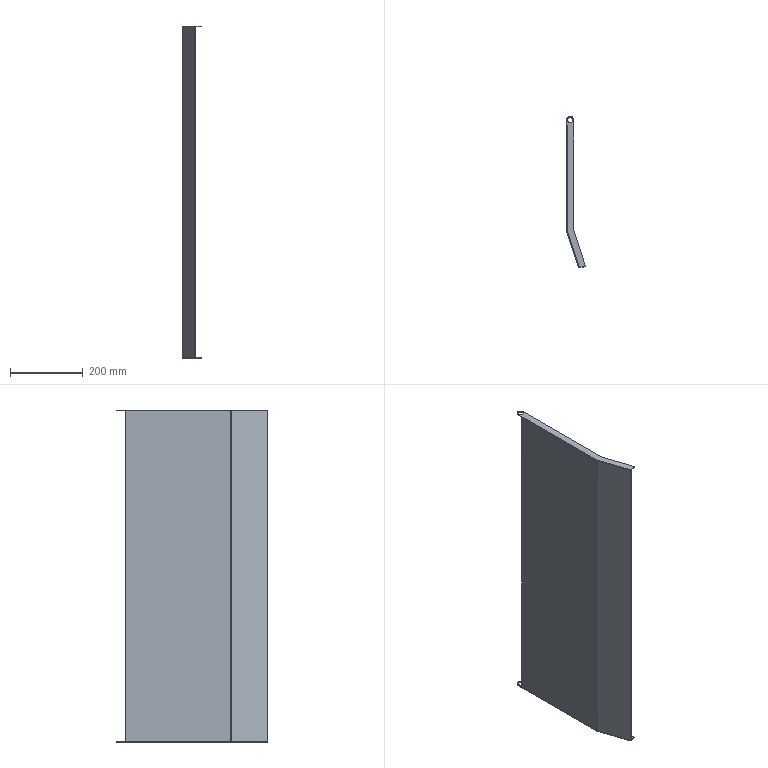Part | SolidWorks | features FlatPattern 2, SMBaseFlange 2, SheetMetal 2, ICE 1, MirrorSolid 1 | 2 solids | 46 faces | box 52.165 x 415.629 x 914 mm | volume 1472368 mm3 | plane 36 | cylinder 10 | commonest cylinder face diameters 15 x4 1.473 x2 5.473 x2 20 x2
STEP:
#1=CARTESIAN_POINT('',(0.5,405.,455.));
#2=VERTEX_POINT('',#1);
#3=CARTESIAN_POINT('',(15.5,405.,455.));
#4=VERTEX_POINT('',#3);
#5=CARTESIAN_POINT('',(8.,405.,455.));
#6=DIRECTION('',(0.,0.,1.));
#7=DIRECTION('',(1.,0.,0.));
#8=AXIS2_PLACEMENT_3D('',#5,#6,#7);
#9=CIRCLE('',#8,7.5);
#10=EDGE_CURVE('',#2,#4,#9,.T.);
#11=ORIENTED_EDGE('',*,*,#10,.F.);
#12=CARTESIAN_POINT('',(0.5,405.,457.));
#13=VERTEX_POINT('',#12);
#14=CARTESIAN_POINT('',(0.5,405.,455.));
#15=DIRECTION('',(0.,0.,1.));
#16=VECTOR('',#15,1000.);
#17=LINE('',#14,#16);
#18=EDGE_CURVE('',#2,#13,#17,.T.);
#19=ORIENTED_EDGE('',*,*,#18,.T.);
#20=CARTESIAN_POINT('',(15.5,405.,457.));
#21=VERTEX_POINT('',#20);
#22=CARTESIAN_POINT('',(8.,405.,457.));
#23=DIRECTION('',(0.,0.,1.));
#24=DIRECTION('',(1.,0.,0.));
#25=AXIS2_PLACEMENT_3D('',#22,#23,#24);
#26=CIRCLE('',#25,7.5);
#27=EDGE_CURVE('',#13,#21,#26,.T.);
#28=ORIENTED_EDGE('',*,*,#27,.T.);
#29=CARTESIAN_POINT('',(15.5,405.,455.));
#30=DIRECTION('',(0.,0.,1.));
#31=VECTOR('',#30,1000.);
#32=LINE('',#29,#31);
#33=EDGE_CURVE('',#4,#21,#32,.T.);
#34=ORIENTED_EDGE('',*,*,#33,.F.);
#35=EDGE_LOOP('',(#11,#19,#28,#34));
#36=FACE_OUTER_BOUND('',#35,.T.);
#37=CARTESIAN_POINT('',(8.,405.,455.));
#38=DIRECTION('',(0.,0.,1.));
#39=DIRECTION('',(1.,0.,0.));
#40=AXIS2_PLACEMENT_3D('',#37,#38,#39);
#41=CYLINDRICAL_SURFACE('',#40,7.5);
#42=ADVANCED_FACE('',(#36),#41,.F.);
#43=CARTESIAN_POINT('',(-2.,390.,455.));
#44=VERTEX_POINT('',#43);
#45=CARTESIAN_POINT('',(-2.,390.,-455.));
#46=VERTEX_POINT('',#45);
#47=CARTESIAN_POINT('',(-2.,390.,455.));
#48=DIRECTION('',(0.,0.,-1.));
#49=VECTOR('',#48,1000.);
#50=LINE('',#47,#49);
#51=EDGE_CURVE('',#44,#46,#50,.T.);
#52=ORIENTED_EDGE('',*,*,#51,.F.);
#53=CARTESIAN_POINT('',(0.,390.,455.));
#54=VERTEX_POINT('',#53);
#55=CARTESIAN_POINT('',(-2.,390.,455.));
#56=DIRECTION('',(1.,0.,0.));
#57=VECTOR('',#56,1000.);
#58=LINE('',#55,#57);
#59=EDGE_CURVE('',#44,#54,#58,.T.);
#60=ORIENTED_EDGE('',*,*,#59,.T.);
#61=CARTESIAN_POINT('',(0.,390.,-455.));
#62=VERTEX_POINT('',#61);
#63=CARTESIAN_POINT('',(0.,390.,455.));
#64=DIRECTION('',(0.,0.,-1.));
#65=VECTOR('',#64,1000.);
#66=LINE('',#63,#65);
#67=EDGE_CURVE('',#54,#62,#66,.T.);
#68=ORIENTED_EDGE('',*,*,#67,.T.);
#69=CARTESIAN_POINT('',(-2.,390.,-455.));
#70=DIRECTION('',(1.,0.,0.));
#71=VECTOR('',#70,1000.);
#72=LINE('',#69,#71);
#73=EDGE_CURVE('',#46,#62,#72,.T.);
#74=ORIENTED_EDGE('',*,*,#73,.F.);
#75=EDGE_LOOP('',(#52,#60,#68,#74));
#76=FACE_OUTER_BOUND('',#75,.T.);
#77=CARTESIAN_POINT('',(-2.,390.,455.));
#78=DIRECTION('',(0.,1.,0.));
#79=DIRECTION('',(0.,0.,1.));
#80=AXIS2_PLACEMENT_3D('',#77,#78,#79);
#81=PLANE('',#80);
#82=ADVANCED_FACE('',(#76),#81,.T.);
#83=CARTESIAN_POINT('',(-2.,100.119,455.));
#84=VERTEX_POINT('',#83);
#85=CARTESIAN_POINT('',(-1.861,99.258,455.));
#86=VERTEX_POINT('',#85);
#87=CARTESIAN_POINT('',(0.7366,100.119,455.));
#88=DIRECTION('',(0.,0.,1.));
#89=DIRECTION('',(1.,0.,0.));
#90=AXIS2_PLACEMENT_3D('',#87,#88,#89);
#91=CIRCLE('',#90,2.737);
#92=EDGE_CURVE('',#84,#86,#91,.T.);
#93=ORIENTED_EDGE('',*,*,#92,.T.);
#94=CARTESIAN_POINT('',(-1.862,100.119,455.));
#95=VERTEX_POINT('',#94);
#96=CARTESIAN_POINT('',(-1.861,99.258,455.));
#97=DIRECTION('',(0.0004776,-1.,0.));
#98=VECTOR('',#97,1000.);
#99=LINE('',#96,#98);
#100=EDGE_CURVE('',#95,#86,#99,.T.);
#101=ORIENTED_EDGE('',*,*,#100,.F.);
#102=CARTESIAN_POINT('',(-2.,100.119,455.));
#103=DIRECTION('',(1.,0.,0.));
#104=VECTOR('',#103,1000.);
#105=LINE('',#102,#104);
#106=EDGE_CURVE('',#84,#95,#105,.T.);
#107=ORIENTED_EDGE('',*,*,#106,.F.);
#108=EDGE_LOOP('',(#93,#101,#107));
#109=FACE_OUTER_BOUND('',#108,.T.);
#110=CARTESIAN_POINT('',(0.03738,99.887,455.));
#111=DIRECTION('',(0.,0.,1.));
#112=DIRECTION('',(1.,0.,0.));
#113=AXIS2_PLACEMENT_3D('',#110,#111,#112);
#114=PLANE('',#113);
#115=ADVANCED_FACE('',(#109),#114,.T.);
#116=CARTESIAN_POINT('',(-1.861,99.258,455.));
#117=DIRECTION('',(0.0004776,-1.,0.));
#118=VECTOR('',#117,1000.);
#119=LINE('',#116,#118);
#120=EDGE_CURVE('',#44,#95,#119,.T.);
#121=ORIENTED_EDGE('',*,*,#120,.F.);
#122=CARTESIAN_POINT('',(-2.,390.,455.));
#123=DIRECTION('',(0.,-1.,0.));
#124=VECTOR('',#123,1000.);
#125=LINE('',#122,#124);
#126=EDGE_CURVE('',#44,#84,#125,.T.);
#127=ORIENTED_EDGE('',*,*,#126,.T.);
#128=ORIENTED_EDGE('',*,*,#106,.T.);
#129=EDGE_LOOP('',(#121,#127,#128));
#130=FACE_OUTER_BOUND('',#129,.T.);
#131=CARTESIAN_POINT('',(0.7366,100.119,455.));
#132=DIRECTION('',(0.,0.,-1.));
#133=DIRECTION('',(-1.,0.,0.));
#134=AXIS2_PLACEMENT_3D('',#131,#132,#133);
#135=PLANE('',#134);
#136=ADVANCED_FACE('',(#130),#135,.F.);
#137=CARTESIAN_POINT('',(0.,100.119,-455.));
#138=VERTEX_POINT('',#137);
#139=CARTESIAN_POINT('',(-2.,100.119,-455.));
#140=VERTEX_POINT('',#139);
#141=CARTESIAN_POINT('',(0.,100.119,-455.));
#142=DIRECTION('',(-1.,0.,0.));
#143=VECTOR('',#142,1000.);
#144=LINE('',#141,#143);
#145=EDGE_CURVE('',#138,#140,#144,.T.);
#146=ORIENTED_EDGE('',*,*,#145,.F.);
#147=CARTESIAN_POINT('',(0.03738,99.887,-455.));
#148=VERTEX_POINT('',#147);
#149=CARTESIAN_POINT('',(0.7366,100.119,-455.));
#150=DIRECTION('',(0.,0.,1.));
#151=DIRECTION('',(-1.,0.,0.));
#152=AXIS2_PLACEMENT_3D('',#149,#150,#151);
#153=CIRCLE('',#152,0.7366);
#154=EDGE_CURVE('',#138,#148,#153,.T.);
#155=ORIENTED_EDGE('',*,*,#154,.T.);
#156=CARTESIAN_POINT('',(-1.861,99.258,-455.));
#157=VERTEX_POINT('',#156);
#158=CARTESIAN_POINT('',(-1.861,99.258,-455.));
#159=DIRECTION('',(0.9493,0.3145,0.));
#160=VECTOR('',#159,1000.);
#161=LINE('',#158,#160);
#162=EDGE_CURVE('',#157,#148,#161,.T.);
#163=ORIENTED_EDGE('',*,*,#162,.F.);
#164=CARTESIAN_POINT('',(0.7366,100.119,-455.));
#165=DIRECTION('',(0.,0.,1.));
#166=DIRECTION('',(1.,0.,0.));
#167=AXIS2_PLACEMENT_3D('',#164,#165,#166);
#168=CIRCLE('',#167,2.737);
#169=EDGE_CURVE('',#140,#157,#168,.T.);
#170=ORIENTED_EDGE('',*,*,#169,.F.);
#171=EDGE_LOOP('',(#146,#155,#163,#170));
#172=FACE_OUTER_BOUND('',#171,.T.);
#173=CARTESIAN_POINT('',(0.,100.119,-455.));
#174=DIRECTION('',(0.,0.,-1.));
#175=DIRECTION('',(-1.,0.,0.));
#176=AXIS2_PLACEMENT_3D('',#173,#174,#175);
#177=PLANE('',#176);
#178=ADVANCED_FACE('',(#172),#177,.T.);
#179=CARTESIAN_POINT('',(0.,390.,-455.));
#180=DIRECTION('',(0.,-1.,0.));
#181=VECTOR('',#180,1000.);
#182=LINE('',#179,#181);
#183=EDGE_CURVE('',#62,#138,#182,.T.);
#184=ORIENTED_EDGE('',*,*,#183,.T.);
#185=ORIENTED_EDGE('',*,*,#145,.T.);
#186=CARTESIAN_POINT('',(-2.,390.,-455.));
#187=DIRECTION('',(0.,-1.,0.));
#188=VECTOR('',#187,1000.);
#189=LINE('',#186,#188);
#190=EDGE_CURVE('',#46,#140,#189,.T.);
#191=ORIENTED_EDGE('',*,*,#190,.F.);
#192=ORIENTED_EDGE('',*,*,#73,.T.);
#193=EDGE_LOOP('',(#184,#185,#191,#192));
#194=FACE_OUTER_BOUND('',#193,.T.);
#195=CARTESIAN_POINT('',(-1.861,99.258,-455.));
#196=DIRECTION('',(0.,0.,-1.));
#197=DIRECTION('',(-1.,0.,0.));
#198=AXIS2_PLACEMENT_3D('',#195,#196,#197);
#199=PLANE('',#198);
#200=ADVANCED_FACE('',(#194),#199,.T.);
#201=CARTESIAN_POINT('',(31.233,-0.629,-455.));
#202=VERTEX_POINT('',#201);
#203=CARTESIAN_POINT('',(-1.899,99.371,-455.));
#204=DIRECTION('',(0.3145,-0.9493,0.));
#205=VECTOR('',#204,1000.);
#206=LINE('',#203,#205);
#207=EDGE_CURVE('',#157,#202,#206,.T.);
#208=ORIENTED_EDGE('',*,*,#207,.T.);
#209=CARTESIAN_POINT('',(31.233,-0.629,455.));
#210=VERTEX_POINT('',#209);
#211=CARTESIAN_POINT('',(31.233,-0.629,455.));
#212=DIRECTION('',(0.,0.,-1.));
#213=VECTOR('',#212,1000.);
#214=LINE('',#211,#213);
#215=EDGE_CURVE('',#210,#202,#214,.T.);
#216=ORIENTED_EDGE('',*,*,#215,.F.);
#217=CARTESIAN_POINT('',(31.233,-0.629,457.));
#218=VERTEX_POINT('',#217);
#219=CARTESIAN_POINT('',(31.233,-0.629,457.));
#220=DIRECTION('',(0.,0.,-1.));
#221=VECTOR('',#220,1000.);
#222=LINE('',#219,#221);
#223=EDGE_CURVE('',#218,#210,#222,.T.);
#224=ORIENTED_EDGE('',*,*,#223,.F.);
#225=CARTESIAN_POINT('',(-1.861,99.258,457.));
#226=VERTEX_POINT('',#225);
#227=CARTESIAN_POINT('',(31.233,-0.629,457.));
#228=DIRECTION('',(0.3145,-0.9493,0.));
#229=VECTOR('',#228,1000.);
#230=LINE('',#227,#229);
#231=EDGE_CURVE('',#226,#218,#230,.T.);
#232=ORIENTED_EDGE('',*,*,#231,.F.);
#233=CARTESIAN_POINT('',(-1.861,99.258,457.));
#234=DIRECTION('',(0.,0.,-1.));
#235=VECTOR('',#234,1000.);
#236=LINE('',#233,#235);
#237=EDGE_CURVE('',#226,#86,#236,.T.);
#238=ORIENTED_EDGE('',*,*,#237,.T.);
#239=CARTESIAN_POINT('',(-1.861,99.258,455.));
#240=DIRECTION('',(0.,0.,-1.));
#241=VECTOR('',#240,1000.);
#242=LINE('',#239,#241);
#243=EDGE_CURVE('',#86,#157,#242,.T.);
#244=ORIENTED_EDGE('',*,*,#243,.T.);
#245=EDGE_LOOP('',(#208,#216,#224,#232,#238,#244));
#246=FACE_OUTER_BOUND('',#245,.T.);
#247=CARTESIAN_POINT('',(-1.899,99.371,455.));
#248=DIRECTION('',(0.9493,0.3145,0.));
#249=DIRECTION('',(-0.3145,0.9493,0.));
#250=AXIS2_PLACEMENT_3D('',#247,#248,#249);
#251=PLANE('',#250);
#252=ADVANCED_FACE('',(#246),#251,.F.);
#253=CARTESIAN_POINT('',(33.132,0.,-455.));
#254=VERTEX_POINT('',#253);
#255=CARTESIAN_POINT('',(33.132,0.,-455.));
#256=DIRECTION('',(-0.9493,-0.3145,0.));
#257=VECTOR('',#256,1000.);
#258=LINE('',#255,#257);
#259=EDGE_CURVE('',#254,#202,#258,.T.);
#260=ORIENTED_EDGE('',*,*,#259,.F.);
#261=CARTESIAN_POINT('',(33.132,0.,455.));
#262=VERTEX_POINT('',#261);
#263=CARTESIAN_POINT('',(33.132,0.,455.));
#264=DIRECTION('',(0.,0.,-1.));
#265=VECTOR('',#264,1000.);
#266=LINE('',#263,#265);
#267=EDGE_CURVE('',#262,#254,#266,.T.);
#268=ORIENTED_EDGE('',*,*,#267,.F.);
#269=CARTESIAN_POINT('',(33.132,0.,455.));
#270=DIRECTION('',(-0.9493,-0.3145,0.));
#271=VECTOR('',#270,1000.);
#272=LINE('',#269,#271);
#273=EDGE_CURVE('',#262,#210,#272,.T.);
#274=ORIENTED_EDGE('',*,*,#273,.T.);
#275=ORIENTED_EDGE('',*,*,#215,.T.);
#276=EDGE_LOOP('',(#260,#268,#274,#275));
#277=FACE_OUTER_BOUND('',#276,.T.);
#278=CARTESIAN_POINT('',(33.132,0.,455.));
#279=DIRECTION('',(0.3145,-0.9493,0.));
#280=DIRECTION('',(0.9493,0.3145,0.));
#281=AXIS2_PLACEMENT_3D('',#278,#279,#280);
#282=PLANE('',#281);
#283=ADVANCED_FACE('',(#277),#282,.T.);
#284=CARTESIAN_POINT('',(0.,100.,-455.));
#285=DIRECTION('',(0.3145,-0.9493,0.));
#286=VECTOR('',#285,1000.);
#287=LINE('',#284,#286);
#288=EDGE_CURVE('',#148,#254,#287,.T.);
#289=ORIENTED_EDGE('',*,*,#288,.F.);
#290=CARTESIAN_POINT('',(0.03738,99.887,455.));
#291=VERTEX_POINT('',#290);
#292=CARTESIAN_POINT('',(0.03738,99.887,455.));
#293=DIRECTION('',(0.,0.,-1.));
#294=VECTOR('',#293,1000.);
#295=LINE('',#292,#294);
#296=EDGE_CURVE('',#291,#148,#295,.T.);
#297=ORIENTED_EDGE('',*,*,#296,.F.);
#298=CARTESIAN_POINT('',(0.,100.,455.));
#299=DIRECTION('',(0.3145,-0.9493,0.));
#300=VECTOR('',#299,1000.);
#301=LINE('',#298,#300);
#302=EDGE_CURVE('',#291,#262,#301,.T.);
#303=ORIENTED_EDGE('',*,*,#302,.T.);
#304=ORIENTED_EDGE('',*,*,#267,.T.);
#305=EDGE_LOOP('',(#289,#297,#303,#304));
#306=FACE_OUTER_BOUND('',#305,.T.);
#307=CARTESIAN_POINT('',(0.,100.,455.));
#308=DIRECTION('',(0.9493,0.3145,0.));
#309=DIRECTION('',(-0.3145,0.9493,0.));
#310=AXIS2_PLACEMENT_3D('',#307,#308,#309);
#311=PLANE('',#310);
#312=ADVANCED_FACE('',(#306),#311,.T.);
#313=ORIENTED_EDGE('',*,*,#154,.F.);
#314=CARTESIAN_POINT('',(0.,100.119,455.));
#315=VERTEX_POINT('',#314);
#316=CARTESIAN_POINT('',(0.,100.119,455.));
#317=DIRECTION('',(0.,0.,-1.));
#318=VECTOR('',#317,1000.);
#319=LINE('',#316,#318);
#320=EDGE_CURVE('',#315,#138,#319,.T.);
#321=ORIENTED_EDGE('',*,*,#320,.F.);
#322=CARTESIAN_POINT('',(0.7366,100.119,455.));
#323=DIRECTION('',(0.,0.,1.));
#324=DIRECTION('',(-1.,0.,0.));
#325=AXIS2_PLACEMENT_3D('',#322,#323,#324);
#326=CIRCLE('',#325,0.7366);
#327=EDGE_CURVE('',#315,#291,#326,.T.);
#328=ORIENTED_EDGE('',*,*,#327,.T.);
#329=ORIENTED_EDGE('',*,*,#296,.T.);
#330=EDGE_LOOP('',(#313,#321,#328,#329));
#331=FACE_OUTER_BOUND('',#330,.T.);
#332=CARTESIAN_POINT('',(0.7366,100.119,455.));
#333=DIRECTION('',(0.,0.,-1.));
#334=DIRECTION('',(-1.,0.,0.));
#335=AXIS2_PLACEMENT_3D('',#332,#333,#334);
#336=CYLINDRICAL_SURFACE('',#335,0.7366);
#337=ADVANCED_FACE('',(#331),#336,.F.);
#338=ORIENTED_EDGE('',*,*,#183,.F.);
#339=ORIENTED_EDGE('',*,*,#67,.F.);
#340=CARTESIAN_POINT('',(0.,390.,455.));
#341=DIRECTION('',(0.,-1.,0.));
#342=VECTOR('',#341,1000.);
#343=LINE('',#340,#342);
#344=EDGE_CURVE('',#54,#315,#343,.T.);
#345=ORIENTED_EDGE('',*,*,#344,.T.);
#346=ORIENTED_EDGE('',*,*,#320,.T.);
#347=EDGE_LOOP('',(#338,#339,#345,#346));
#348=FACE_OUTER_BOUND('',#347,.T.);
#349=CARTESIAN_POINT('',(0.,390.,455.));
#350=DIRECTION('',(1.,0.,0.));
#351=DIRECTION('',(0.,1.,0.));
#352=AXIS2_PLACEMENT_3D('',#349,#350,#351);
#353=PLANE('',#352);
#354=ADVANCED_FACE('',(#348),#353,.T.);
#355=ORIENTED_EDGE('',*,*,#190,.T.);
#356=CARTESIAN_POINT('',(-2.,100.119,455.));
#357=DIRECTION('',(0.,0.,-1.));
#358=VECTOR('',#357,1000.);
#359=LINE('',#356,#358);
#360=EDGE_CURVE('',#84,#140,#359,.T.);
#361=ORIENTED_EDGE('',*,*,#360,.F.);
#362=ORIENTED_EDGE('',*,*,#126,.F.);
#363=ORIENTED_EDGE('',*,*,#51,.T.);
#364=EDGE_LOOP('',(#355,#361,#362,#363));
#365=FACE_OUTER_BOUND('',#364,.T.);
#366=CARTESIAN_POINT('',(-2.,390.,455.));
#367=DIRECTION('',(1.,0.,0.));
#368=DIRECTION('',(0.,1.,0.));
#369=AXIS2_PLACEMENT_3D('',#366,#367,#368);
#370=PLANE('',#369);
#371=ADVANCED_FACE('',(#365),#370,.F.);
#372=ORIENTED_EDGE('',*,*,#169,.T.);
#373=ORIENTED_EDGE('',*,*,#243,.F.);
#374=ORIENTED_EDGE('',*,*,#92,.F.);
#375=ORIENTED_EDGE('',*,*,#360,.T.);
#376=EDGE_LOOP('',(#372,#373,#374,#375));
#377=FACE_OUTER_BOUND('',#376,.T.);
#378=CARTESIAN_POINT('',(0.7366,100.119,455.));
#379=DIRECTION('',(0.,0.,-1.));
#380=DIRECTION('',(-1.,0.,0.));
#381=AXIS2_PLACEMENT_3D('',#378,#379,#380);
#382=CYLINDRICAL_SURFACE('',#381,2.737);
#383=ADVANCED_FACE('',(#377),#382,.T.);
#384=ORIENTED_EDGE('',*,*,#207,.F.);
#385=ORIENTED_EDGE('',*,*,#162,.T.);
#386=ORIENTED_EDGE('',*,*,#288,.T.);
#387=ORIENTED_EDGE('',*,*,#259,.T.);
#388=EDGE_LOOP('',(#384,#385,#386,#387));
#389=FACE_OUTER_BOUND('',#388,.T.);
#390=CARTESIAN_POINT('',(0.7366,100.119,-455.));
#391=DIRECTION('',(0.,0.,-1.));
#392=DIRECTION('',(-1.,0.,0.));
#393=AXIS2_PLACEMENT_3D('',#390,#391,#392);
#394=PLANE('',#393);
#395=ADVANCED_FACE('',(#389),#394,.T.);
#396=ORIENTED_EDGE('',*,*,#273,.F.);
#397=ORIENTED_EDGE('',*,*,#302,.F.);
#398=ORIENTED_EDGE('',*,*,#327,.F.);
#399=ORIENTED_EDGE('',*,*,#344,.F.);
#400=ORIENTED_EDGE('',*,*,#59,.F.);
#401=CARTESIAN_POINT('',(-2.,405.,455.));
#402=VERTEX_POINT('',#401);
#403=CARTESIAN_POINT('',(-2.,390.,455.));
#404=DIRECTION('',(0.,-1.,0.));
#405=VECTOR('',#404,1000.);
#406=LINE('',#403,#405);
#407=EDGE_CURVE('',#402,#44,#406,.T.);
#408=ORIENTED_EDGE('',*,*,#407,.F.);
#409=CARTESIAN_POINT('',(18.,405.,455.));
#410=VERTEX_POINT('',#409);
#411=CARTESIAN_POINT('',(8.,405.,455.));
#412=DIRECTION('',(0.,0.,1.));
#413=DIRECTION('',(1.,0.,0.));
#414=AXIS2_PLACEMENT_3D('',#411,#412,#413);
#415=CIRCLE('',#414,10.);
#416=EDGE_CURVE('',#410,#402,#415,.T.);
#417=ORIENTED_EDGE('',*,*,#416,.F.);
#418=CARTESIAN_POINT('',(18.,99.573,455.));
#419=VERTEX_POINT('',#418);
#420=CARTESIAN_POINT('',(18.,390.,455.));
#421=DIRECTION('',(0.,1.,0.));
#422=VECTOR('',#421,1000.);
#423=LINE('',#420,#422);
#424=EDGE_CURVE('',#419,#410,#423,.T.);
#425=ORIENTED_EDGE('',*,*,#424,.F.);
#426=CARTESIAN_POINT('',(50.165,2.49,455.));
#427=VERTEX_POINT('',#426);
#428=CARTESIAN_POINT('',(18.,99.573,455.));
#429=DIRECTION('',(-0.3145,0.9493,0.));
#430=VECTOR('',#429,1000.);
#431=LINE('',#428,#430);
#432=EDGE_CURVE('',#427,#419,#431,.T.);
#433=ORIENTED_EDGE('',*,*,#432,.F.);
#434=CARTESIAN_POINT('',(50.165,2.49,455.));
#435=DIRECTION('',(0.9867,0.1625,0.));
#436=VECTOR('',#435,1000.);
#437=LINE('',#434,#436);
#438=EDGE_CURVE('',#210,#427,#437,.T.);
#439=ORIENTED_EDGE('',*,*,#438,.F.);
#440=EDGE_LOOP('',(#396,#397,#398,#399,#400,#408,#417,#425,#433,#439));
#441=FACE_OUTER_BOUND('',#440,.T.);
#442=CARTESIAN_POINT('',(8.,405.,455.));
#443=DIRECTION('',(0.,0.,1.));
#444=DIRECTION('',(1.,0.,0.));
#445=AXIS2_PLACEMENT_3D('',#442,#443,#444);
#446=CIRCLE('',#445,7.5);
#447=EDGE_CURVE('',#4,#2,#446,.T.);
#448=ORIENTED_EDGE('',*,*,#447,.T.);
#449=ORIENTED_EDGE('',*,*,#10,.T.);
#450=EDGE_LOOP('',(#448,#449));
#451=FACE_BOUND('',#450,.T.);
#452=CARTESIAN_POINT('',(0.,0.,455.));
#453=DIRECTION('',(0.,0.,1.));
#454=DIRECTION('',(1.,0.,0.));
#455=AXIS2_PLACEMENT_3D('',#452,#453,#454);
#456=PLANE('',#455);
#457=ADVANCED_FACE('',(#441,#451),#456,.F.);
#458=ORIENTED_EDGE('',*,*,#424,.T.);
#459=CARTESIAN_POINT('',(18.,405.,457.));
#460=VERTEX_POINT('',#459);
#461=CARTESIAN_POINT('',(18.,405.,455.));
#462=DIRECTION('',(0.,0.,1.));
#463=VECTOR('',#462,1000.);
#464=LINE('',#461,#463);
#465=EDGE_CURVE('',#410,#460,#464,.T.);
#466=ORIENTED_EDGE('',*,*,#465,.T.);
#467=CARTESIAN_POINT('',(18.,99.573,457.));
#468=VERTEX_POINT('',#467);
#469=CARTESIAN_POINT('',(18.,390.,457.));
#470=DIRECTION('',(0.,1.,0.));
#471=VECTOR('',#470,1000.);
#472=LINE('',#469,#471);
#473=EDGE_CURVE('',#468,#460,#472,.T.);
#474=ORIENTED_EDGE('',*,*,#473,.F.);
#475=CARTESIAN_POINT('',(18.,99.573,457.));
#476=DIRECTION('',(0.,0.,-1.));
#477=VECTOR('',#476,1000.);
#478=LINE('',#475,#477);
#479=EDGE_CURVE('',#468,#419,#478,.T.);
#480=ORIENTED_EDGE('',*,*,#479,.T.);
#481=EDGE_LOOP('',(#458,#466,#474,#480));
#482=FACE_OUTER_BOUND('',#481,.T.);
#483=CARTESIAN_POINT('',(18.,390.,457.));
#484=DIRECTION('',(-1.,0.,0.));
#485=DIRECTION('',(0.,-1.,0.));
#486=AXIS2_PLACEMENT_3D('',#483,#484,#485);
#487=PLANE('',#486);
#488=ADVANCED_FACE('',(#482),#487,.F.);
#489=ORIENTED_EDGE('',*,*,#120,.T.);
#490=ORIENTED_EDGE('',*,*,#100,.T.);
#491=ORIENTED_EDGE('',*,*,#237,.F.);
#492=CARTESIAN_POINT('',(-2.,390.,457.));
#493=VERTEX_POINT('',#492);
#494=CARTESIAN_POINT('',(-1.861,99.258,457.));
#495=DIRECTION('',(0.0004776,-1.,0.));
#496=VECTOR('',#495,1000.);
#497=LINE('',#494,#496);
#498=EDGE_CURVE('',#493,#226,#497,.T.);
#499=ORIENTED_EDGE('',*,*,#498,.F.);
#500=CARTESIAN_POINT('',(-2.,390.,457.));
#501=DIRECTION('',(0.,0.,-1.));
#502=VECTOR('',#501,1000.);
#503=LINE('',#500,#502);
#504=EDGE_CURVE('',#493,#44,#503,.T.);
#505=ORIENTED_EDGE('',*,*,#504,.T.);
#506=EDGE_LOOP('',(#489,#490,#491,#499,#505));
#507=FACE_OUTER_BOUND('',#506,.T.);
#508=CARTESIAN_POINT('',(-1.861,99.258,457.));
#509=DIRECTION('',(1.,0.0004776,0.));
#510=DIRECTION('',(-0.0004776,1.,0.));
#511=AXIS2_PLACEMENT_3D('',#508,#509,#510);
#512=PLANE('',#511);
#513=ADVANCED_FACE('',(#507),#512,.F.);
#514=ORIENTED_EDGE('',*,*,#438,.T.);
#515=CARTESIAN_POINT('',(50.165,2.49,457.));
#516=VERTEX_POINT('',#515);
#517=CARTESIAN_POINT('',(50.165,2.49,457.));
#518=DIRECTION('',(0.,0.,-1.));
#519=VECTOR('',#518,1000.);
#520=LINE('',#517,#519);
#521=EDGE_CURVE('',#516,#427,#520,.T.);
#522=ORIENTED_EDGE('',*,*,#521,.F.);
#523=CARTESIAN_POINT('',(50.165,2.49,457.));
#524=DIRECTION('',(0.9867,0.1625,0.));
#525=VECTOR('',#524,1000.);
#526=LINE('',#523,#525);
#527=EDGE_CURVE('',#218,#516,#526,.T.);
#528=ORIENTED_EDGE('',*,*,#527,.F.);
#529=ORIENTED_EDGE('',*,*,#223,.T.);
#530=EDGE_LOOP('',(#514,#522,#528,#529));
#531=FACE_OUTER_BOUND('',#530,.T.);
#532=CARTESIAN_POINT('',(50.165,2.49,457.));
#533=DIRECTION('',(-0.1625,0.9867,0.));
#534=DIRECTION('',(-0.9867,-0.1625,0.));
#535=AXIS2_PLACEMENT_3D('',#532,#533,#534);
#536=PLANE('',#535);
#537=ADVANCED_FACE('',(#531),#536,.F.);
#538=ORIENTED_EDGE('',*,*,#432,.T.);
#539=ORIENTED_EDGE('',*,*,#479,.F.);
#540=CARTESIAN_POINT('',(18.,99.573,457.));
#541=DIRECTION('',(-0.3145,0.9493,0.));
#542=VECTOR('',#541,1000.);
#543=LINE('',#540,#542);
#544=EDGE_CURVE('',#516,#468,#543,.T.);
#545=ORIENTED_EDGE('',*,*,#544,.F.);
#546=ORIENTED_EDGE('',*,*,#521,.T.);
#547=EDGE_LOOP('',(#538,#539,#545,#546));
#548=FACE_OUTER_BOUND('',#547,.T.);
#549=CARTESIAN_POINT('',(18.,99.573,457.));
#550=DIRECTION('',(-0.9493,-0.3145,0.));
#551=DIRECTION('',(0.3145,-0.9493,0.));
#552=AXIS2_PLACEMENT_3D('',#549,#550,#551);
#553=PLANE('',#552);
#554=ADVANCED_FACE('',(#548),#553,.F.);
#555=ORIENTED_EDGE('',*,*,#473,.T.);
#556=CARTESIAN_POINT('',(-2.,405.,457.));
#557=VERTEX_POINT('',#556);
#558=CARTESIAN_POINT('',(8.,405.,457.));
#559=DIRECTION('',(0.,0.,1.));
#560=DIRECTION('',(1.,0.,0.));
#561=AXIS2_PLACEMENT_3D('',#558,#559,#560);
#562=CIRCLE('',#561,10.);
#563=EDGE_CURVE('',#460,#557,#562,.T.);
#564=ORIENTED_EDGE('',*,*,#563,.T.);
#565=CARTESIAN_POINT('',(-2.,390.,457.));
#566=DIRECTION('',(0.,-1.,0.));
#567=VECTOR('',#566,1000.);
#568=LINE('',#565,#567);
#569=EDGE_CURVE('',#557,#493,#568,.T.);
#570=ORIENTED_EDGE('',*,*,#569,.T.);
#571=ORIENTED_EDGE('',*,*,#498,.T.);
#572=ORIENTED_EDGE('',*,*,#231,.T.);
#573=ORIENTED_EDGE('',*,*,#527,.T.);
#574=ORIENTED_EDGE('',*,*,#544,.T.);
#575=EDGE_LOOP('',(#555,#564,#570,#571,#572,#573,#574));
#576=FACE_OUTER_BOUND('',#575,.T.);
#577=CARTESIAN_POINT('',(8.,405.,457.));
#578=DIRECTION('',(0.,0.,1.));
#579=DIRECTION('',(1.,0.,0.));
#580=AXIS2_PLACEMENT_3D('',#577,#578,#579);
#581=CIRCLE('',#580,7.5);
#582=EDGE_CURVE('',#21,#13,#581,.T.);
#583=ORIENTED_EDGE('',*,*,#582,.F.);
#584=ORIENTED_EDGE('',*,*,#27,.F.);
#585=EDGE_LOOP('',(#583,#584));
#586=FACE_BOUND('',#585,.T.);
#587=CARTESIAN_POINT('',(0.,0.,457.));
#588=DIRECTION('',(0.,0.,1.));
#589=DIRECTION('',(1.,0.,0.));
#590=AXIS2_PLACEMENT_3D('',#587,#588,#589);
#591=PLANE('',#590);
#592=ADVANCED_FACE('',(#576,#586),#591,.T.);
#593=ORIENTED_EDGE('',*,*,#569,.F.);
#594=CARTESIAN_POINT('',(-2.,405.,455.));
#595=DIRECTION('',(0.,0.,1.));
#596=VECTOR('',#595,1000.);
#597=LINE('',#594,#596);
#598=EDGE_CURVE('',#402,#557,#597,.T.);
#599=ORIENTED_EDGE('',*,*,#598,.F.);
#600=ORIENTED_EDGE('',*,*,#407,.T.);
#601=ORIENTED_EDGE('',*,*,#504,.F.);
#602=EDGE_LOOP('',(#593,#599,#600,#601));
#603=FACE_OUTER_BOUND('',#602,.T.);
#604=CARTESIAN_POINT('',(-2.,390.,455.));
#605=DIRECTION('',(-1.,0.,0.));
#606=DIRECTION('',(0.,0.,1.));
#607=AXIS2_PLACEMENT_3D('',#604,#605,#606);
#608=PLANE('',#607);
#609=ADVANCED_FACE('',(#603),#608,.T.);
#610=ORIENTED_EDGE('',*,*,#563,.F.);
#611=ORIENTED_EDGE('',*,*,#465,.F.);
#612=ORIENTED_EDGE('',*,*,#416,.T.);
#613=ORIENTED_EDGE('',*,*,#598,.T.);
#614=EDGE_LOOP('',(#610,#611,#612,#613));
#615=FACE_OUTER_BOUND('',#614,.T.);
#616=CARTESIAN_POINT('',(8.,405.,455.));
#617=DIRECTION('',(0.,0.,1.));
#618=DIRECTION('',(1.,0.,0.));
#619=AXIS2_PLACEMENT_3D('',#616,#617,#618);
#620=CYLINDRICAL_SURFACE('',#619,10.);
#621=ADVANCED_FACE('',(#615),#620,.T.);
#622=ORIENTED_EDGE('',*,*,#18,.F.);
#623=ORIENTED_EDGE('',*,*,#447,.F.);
#624=ORIENTED_EDGE('',*,*,#33,.T.);
#625=ORIENTED_EDGE('',*,*,#582,.T.);
#626=EDGE_LOOP('',(#622,#623,#624,#625));
#627=FACE_OUTER_BOUND('',#626,.T.);
#628=CARTESIAN_POINT('',(8.,405.,455.));
#629=DIRECTION('',(0.,0.,1.));
#630=DIRECTION('',(1.,0.,0.));
#631=AXIS2_PLACEMENT_3D('',#628,#629,#630);
#632=CYLINDRICAL_SURFACE('',#631,7.5);
#633=ADVANCED_FACE('',(#627),#632,.F.);
#634=CLOSED_SHELL('',(#42,#82,#115,#136,#178,#200,#252,#283,#312,#337,#354,#371,#383,#395,#457,#488,#513,#537,#554,#592,#609,#621,#633));
#635=MANIFOLD_SOLID_BREP('',#634);
#636=CARTESIAN_POINT('',(15.5,405.,-455.));
#637=VERTEX_POINT('',#636);
#638=CARTESIAN_POINT('',(0.5,405.,-455.));
#639=VERTEX_POINT('',#638);
#640=CARTESIAN_POINT('',(8.,405.,-455.));
#641=DIRECTION('',(0.,0.,1.));
#642=DIRECTION('',(1.,0.,0.));
#643=AXIS2_PLACEMENT_3D('',#640,#641,#642);
#644=CIRCLE('',#643,7.5);
#645=EDGE_CURVE('',#637,#639,#644,.T.);
#646=ORIENTED_EDGE('',*,*,#645,.T.);
#647=CARTESIAN_POINT('',(0.5,405.,-457.));
#648=VERTEX_POINT('',#647);
#649=CARTESIAN_POINT('',(0.5,405.,-455.));
#650=DIRECTION('',(0.,0.,-1.));
#651=VECTOR('',#650,1000.);
#652=LINE('',#649,#651);
#653=EDGE_CURVE('',#639,#648,#652,.T.);
#654=ORIENTED_EDGE('',*,*,#653,.T.);
#655=CARTESIAN_POINT('',(15.5,405.,-457.));
#656=VERTEX_POINT('',#655);
#657=CARTESIAN_POINT('',(8.,405.,-457.));
#658=DIRECTION('',(0.,0.,1.));
#659=DIRECTION('',(1.,0.,0.));
#660=AXIS2_PLACEMENT_3D('',#657,#658,#659);
#661=CIRCLE('',#660,7.5);
#662=EDGE_CURVE('',#656,#648,#661,.T.);
#663=ORIENTED_EDGE('',*,*,#662,.F.);
#664=CARTESIAN_POINT('',(15.5,405.,-455.));
#665=DIRECTION('',(0.,0.,-1.));
#666=VECTOR('',#665,1000.);
#667=LINE('',#664,#666);
#668=EDGE_CURVE('',#637,#656,#667,.T.);
#669=ORIENTED_EDGE('',*,*,#668,.F.);
#670=EDGE_LOOP('',(#646,#654,#663,#669));
#671=FACE_OUTER_BOUND('',#670,.T.);
#672=CARTESIAN_POINT('',(8.,405.,-455.));
#673=DIRECTION('',(0.,0.,-1.));
#674=DIRECTION('',(1.,0.,0.));
#675=AXIS2_PLACEMENT_3D('',#672,#673,#674);
#676=CYLINDRICAL_SURFACE('',#675,7.5);
#677=ADVANCED_FACE('',(#671),#676,.F.);
#678=CARTESIAN_POINT('',(-2.,390.,-455.));
#679=VERTEX_POINT('',#678);
#680=CARTESIAN_POINT('',(-2.,390.,455.));
#681=VERTEX_POINT('',#680);
#682=CARTESIAN_POINT('',(-2.,390.,-455.));
#683=DIRECTION('',(0.,0.,1.));
#684=VECTOR('',#683,1000.);
#685=LINE('',#682,#684);
#686=EDGE_CURVE('',#679,#681,#685,.T.);
#687=ORIENTED_EDGE('',*,*,#686,.T.);
#688=CARTESIAN_POINT('',(0.,390.,455.));
#689=VERTEX_POINT('',#688);
#690=CARTESIAN_POINT('',(-2.,390.,455.));
#691=DIRECTION('',(1.,0.,0.));
#692=VECTOR('',#691,1000.);
#693=LINE('',#690,#692);
#694=EDGE_CURVE('',#681,#689,#693,.T.);
#695=ORIENTED_EDGE('',*,*,#694,.T.);
#696=CARTESIAN_POINT('',(0.,390.,-455.));
#697=VERTEX_POINT('',#696);
#698=CARTESIAN_POINT('',(0.,390.,-455.));
#699=DIRECTION('',(0.,0.,1.));
#700=VECTOR('',#699,1000.);
#701=LINE('',#698,#700);
#702=EDGE_CURVE('',#697,#689,#701,.T.);
#703=ORIENTED_EDGE('',*,*,#702,.F.);
#704=CARTESIAN_POINT('',(-2.,390.,-455.));
#705=DIRECTION('',(1.,0.,0.));
#706=VECTOR('',#705,1000.);
#707=LINE('',#704,#706);
#708=EDGE_CURVE('',#679,#697,#707,.T.);
#709=ORIENTED_EDGE('',*,*,#708,.F.);
#710=EDGE_LOOP('',(#687,#695,#703,#709));
#711=FACE_OUTER_BOUND('',#710,.T.);
#712=CARTESIAN_POINT('',(-2.,390.,-455.));
#713=DIRECTION('',(0.,1.,0.));
#714=DIRECTION('',(0.,0.,-1.));
#715=AXIS2_PLACEMENT_3D('',#712,#713,#714);
#716=PLANE('',#715);
#717=ADVANCED_FACE('',(#711),#716,.T.);
#718=CARTESIAN_POINT('',(-2.,100.119,-455.));
#719=VERTEX_POINT('',#718);
#720=CARTESIAN_POINT('',(-1.861,99.258,-455.));
#721=VERTEX_POINT('',#720);
#722=CARTESIAN_POINT('',(0.7366,100.119,-455.));
#723=DIRECTION('',(0.,0.,1.));
#724=DIRECTION('',(1.,0.,0.));
#725=AXIS2_PLACEMENT_3D('',#722,#723,#724);
#726=CIRCLE('',#725,2.737);
#727=EDGE_CURVE('',#719,#721,#726,.T.);
#728=ORIENTED_EDGE('',*,*,#727,.F.);
#729=CARTESIAN_POINT('',(-1.862,100.119,-455.));
#730=VERTEX_POINT('',#729);
#731=CARTESIAN_POINT('',(-2.,100.119,-455.));
#732=DIRECTION('',(1.,0.,0.));
#733=VECTOR('',#732,1000.);
#734=LINE('',#731,#733);
#735=EDGE_CURVE('',#719,#730,#734,.T.);
#736=ORIENTED_EDGE('',*,*,#735,.T.);
#737=CARTESIAN_POINT('',(-1.861,99.258,-455.));
#738=DIRECTION('',(0.0004776,-1.,0.));
#739=VECTOR('',#738,1000.);
#740=LINE('',#737,#739);
#741=EDGE_CURVE('',#730,#721,#740,.T.);
#742=ORIENTED_EDGE('',*,*,#741,.T.);
#743=EDGE_LOOP('',(#728,#736,#742));
#744=FACE_OUTER_BOUND('',#743,.T.);
#745=CARTESIAN_POINT('',(0.03738,99.887,-455.));
#746=DIRECTION('',(0.,0.,-1.));
#747=DIRECTION('',(1.,0.,0.));
#748=AXIS2_PLACEMENT_3D('',#745,#746,#747);
#749=PLANE('',#748);
#750=ADVANCED_FACE('',(#744),#749,.T.);
#751=CARTESIAN_POINT('',(-1.861,99.258,-455.));
#752=DIRECTION('',(0.0004776,-1.,0.));
#753=VECTOR('',#752,1000.);
#754=LINE('',#751,#753);
#755=EDGE_CURVE('',#679,#730,#754,.T.);
#756=ORIENTED_EDGE('',*,*,#755,.T.);
#757=ORIENTED_EDGE('',*,*,#735,.F.);
#758=CARTESIAN_POINT('',(-2.,390.,-455.));
#759=DIRECTION('',(0.,-1.,0.));
#760=VECTOR('',#759,1000.);
#761=LINE('',#758,#760);
#762=EDGE_CURVE('',#679,#719,#761,.T.);
#763=ORIENTED_EDGE('',*,*,#762,.F.);
#764=EDGE_LOOP('',(#756,#757,#763));
#765=FACE_OUTER_BOUND('',#764,.T.);
#766=CARTESIAN_POINT('',(0.7366,100.119,-455.));
#767=DIRECTION('',(0.,0.,1.));
#768=DIRECTION('',(-1.,0.,0.));
#769=AXIS2_PLACEMENT_3D('',#766,#767,#768);
#770=PLANE('',#769);
#771=ADVANCED_FACE('',(#765),#770,.F.);
#772=CARTESIAN_POINT('',(0.,100.119,455.));
#773=VERTEX_POINT('',#772);
#774=CARTESIAN_POINT('',(-2.,100.119,455.));
#775=VERTEX_POINT('',#774);
#776=CARTESIAN_POINT('',(0.,100.119,455.));
#777=DIRECTION('',(-1.,0.,0.));
#778=VECTOR('',#777,1000.);
#779=LINE('',#776,#778);
#780=EDGE_CURVE('',#773,#775,#779,.T.);
#781=ORIENTED_EDGE('',*,*,#780,.T.);
#782=CARTESIAN_POINT('',(-1.861,99.258,455.));
#783=VERTEX_POINT('',#782);
#784=CARTESIAN_POINT('',(0.7366,100.119,455.));
#785=DIRECTION('',(0.,0.,1.));
#786=DIRECTION('',(1.,0.,0.));
#787=AXIS2_PLACEMENT_3D('',#784,#785,#786);
#788=CIRCLE('',#787,2.737);
#789=EDGE_CURVE('',#775,#783,#788,.T.);
#790=ORIENTED_EDGE('',*,*,#789,.T.);
#791=CARTESIAN_POINT('',(0.03738,99.887,455.));
#792=VERTEX_POINT('',#791);
#793=CARTESIAN_POINT('',(-1.861,99.258,455.));
#794=DIRECTION('',(0.9493,0.3145,0.));
#795=VECTOR('',#794,1000.);
#796=LINE('',#793,#795);
#797=EDGE_CURVE('',#783,#792,#796,.T.);
#798=ORIENTED_EDGE('',*,*,#797,.T.);
#799=CARTESIAN_POINT('',(0.7366,100.119,455.));
#800=DIRECTION('',(0.,0.,1.));
#801=DIRECTION('',(-1.,0.,0.));
#802=AXIS2_PLACEMENT_3D('',#799,#800,#801);
#803=CIRCLE('',#802,0.7366);
#804=EDGE_CURVE('',#773,#792,#803,.T.);
#805=ORIENTED_EDGE('',*,*,#804,.F.);
#806=EDGE_LOOP('',(#781,#790,#798,#805));
#807=FACE_OUTER_BOUND('',#806,.T.);
#808=CARTESIAN_POINT('',(0.,100.119,455.));
#809=DIRECTION('',(0.,0.,1.));
#810=DIRECTION('',(-1.,0.,0.));
#811=AXIS2_PLACEMENT_3D('',#808,#809,#810);
#812=PLANE('',#811);
#813=ADVANCED_FACE('',(#807),#812,.T.);
#814=CARTESIAN_POINT('',(0.,390.,455.));
#815=DIRECTION('',(0.,-1.,0.));
#816=VECTOR('',#815,1000.);
#817=LINE('',#814,#816);
#818=EDGE_CURVE('',#689,#773,#817,.T.);
#819=ORIENTED_EDGE('',*,*,#818,.F.);
#820=ORIENTED_EDGE('',*,*,#694,.F.);
#821=CARTESIAN_POINT('',(-2.,390.,455.));
#822=DIRECTION('',(0.,-1.,0.));
#823=VECTOR('',#822,1000.);
#824=LINE('',#821,#823);
#825=EDGE_CURVE('',#681,#775,#824,.T.);
#826=ORIENTED_EDGE('',*,*,#825,.T.);
#827=ORIENTED_EDGE('',*,*,#780,.F.);
#828=EDGE_LOOP('',(#819,#820,#826,#827));
#829=FACE_OUTER_BOUND('',#828,.T.);
#830=CARTESIAN_POINT('',(-1.861,99.258,455.));
#831=DIRECTION('',(0.,0.,1.));
#832=DIRECTION('',(-1.,0.,0.));
#833=AXIS2_PLACEMENT_3D('',#830,#831,#832);
#834=PLANE('',#833);
#835=ADVANCED_FACE('',(#829),#834,.T.);
#836=CARTESIAN_POINT('',(31.233,-0.629,455.));
#837=VERTEX_POINT('',#836);
#838=CARTESIAN_POINT('',(-1.899,99.371,455.));
#839=DIRECTION('',(0.3145,-0.9493,0.));
#840=VECTOR('',#839,1000.);
#841=LINE('',#838,#840);
#842=EDGE_CURVE('',#783,#837,#841,.T.);
#843=ORIENTED_EDGE('',*,*,#842,.F.);
#844=CARTESIAN_POINT('',(-1.861,99.258,-455.));
#845=DIRECTION('',(0.,0.,1.));
#846=VECTOR('',#845,1000.);
#847=LINE('',#844,#846);
#848=EDGE_CURVE('',#721,#783,#847,.T.);
#849=ORIENTED_EDGE('',*,*,#848,.F.);
#850=CARTESIAN_POINT('',(-1.861,99.258,-457.));
#851=VERTEX_POINT('',#850);
#852=CARTESIAN_POINT('',(-1.861,99.258,-457.));
#853=DIRECTION('',(0.,0.,1.));
#854=VECTOR('',#853,1000.);
#855=LINE('',#852,#854);
#856=EDGE_CURVE('',#851,#721,#855,.T.);
#857=ORIENTED_EDGE('',*,*,#856,.F.);
#858=CARTESIAN_POINT('',(31.233,-0.629,-457.));
#859=VERTEX_POINT('',#858);
#860=CARTESIAN_POINT('',(31.233,-0.629,-457.));
#861=DIRECTION('',(0.3145,-0.9493,0.));
#862=VECTOR('',#861,1000.);
#863=LINE('',#860,#862);
#864=EDGE_CURVE('',#851,#859,#863,.T.);
#865=ORIENTED_EDGE('',*,*,#864,.T.);
#866=CARTESIAN_POINT('',(31.233,-0.629,-455.));
#867=VERTEX_POINT('',#866);
#868=CARTESIAN_POINT('',(31.233,-0.629,-457.));
#869=DIRECTION('',(0.,0.,1.));
#870=VECTOR('',#869,1000.);
#871=LINE('',#868,#870);
#872=EDGE_CURVE('',#859,#867,#871,.T.);
#873=ORIENTED_EDGE('',*,*,#872,.T.);
#874=CARTESIAN_POINT('',(31.233,-0.629,-455.));
#875=DIRECTION('',(0.,0.,1.));
#876=VECTOR('',#875,1000.);
#877=LINE('',#874,#876);
#878=EDGE_CURVE('',#867,#837,#877,.T.);
#879=ORIENTED_EDGE('',*,*,#878,.T.);
#880=EDGE_LOOP('',(#843,#849,#857,#865,#873,#879));
#881=FACE_OUTER_BOUND('',#880,.T.);
#882=CARTESIAN_POINT('',(-1.899,99.371,-455.));
#883=DIRECTION('',(0.9493,0.3145,0.));
#884=DIRECTION('',(-0.3145,0.9493,0.));
#885=AXIS2_PLACEMENT_3D('',#882,#883,#884);
#886=PLANE('',#885);
#887=ADVANCED_FACE('',(#881),#886,.F.);
#888=CARTESIAN_POINT('',(33.132,0.,455.));
#889=VERTEX_POINT('',#888);
#890=CARTESIAN_POINT('',(33.132,0.,455.));
#891=DIRECTION('',(-0.9493,-0.3145,0.));
#892=VECTOR('',#891,1000.);
#893=LINE('',#890,#892);
#894=EDGE_CURVE('',#889,#837,#893,.T.);
#895=ORIENTED_EDGE('',*,*,#894,.T.);
#896=ORIENTED_EDGE('',*,*,#878,.F.);
#897=CARTESIAN_POINT('',(33.132,0.,-455.));
#898=VERTEX_POINT('',#897);
#899=CARTESIAN_POINT('',(33.132,0.,-455.));
#900=DIRECTION('',(-0.9493,-0.3145,0.));
#901=VECTOR('',#900,1000.);
#902=LINE('',#899,#901);
#903=EDGE_CURVE('',#898,#867,#902,.T.);
#904=ORIENTED_EDGE('',*,*,#903,.F.);
#905=CARTESIAN_POINT('',(33.132,0.,-455.));
#906=DIRECTION('',(0.,0.,1.));
#907=VECTOR('',#906,1000.);
#908=LINE('',#905,#907);
#909=EDGE_CURVE('',#898,#889,#908,.T.);
#910=ORIENTED_EDGE('',*,*,#909,.T.);
#911=EDGE_LOOP('',(#895,#896,#904,#910));
#912=FACE_OUTER_BOUND('',#911,.T.);
#913=CARTESIAN_POINT('',(33.132,0.,-455.));
#914=DIRECTION('',(0.3145,-0.9493,0.));
#915=DIRECTION('',(0.9493,0.3145,0.));
#916=AXIS2_PLACEMENT_3D('',#913,#914,#915);
#917=PLANE('',#916);
#918=ADVANCED_FACE('',(#912),#917,.T.);
#919=CARTESIAN_POINT('',(0.,100.,455.));
#920=DIRECTION('',(0.3145,-0.9493,0.));
#921=VECTOR('',#920,1000.);
#922=LINE('',#919,#921);
#923=EDGE_CURVE('',#792,#889,#922,.T.);
#924=ORIENTED_EDGE('',*,*,#923,.T.);
#925=ORIENTED_EDGE('',*,*,#909,.F.);
#926=CARTESIAN_POINT('',(0.03738,99.887,-455.));
#927=VERTEX_POINT('',#926);
#928=CARTESIAN_POINT('',(0.,100.,-455.));
#929=DIRECTION('',(0.3145,-0.9493,0.));
#930=VECTOR('',#929,1000.);
#931=LINE('',#928,#930);
#932=EDGE_CURVE('',#927,#898,#931,.T.);
#933=ORIENTED_EDGE('',*,*,#932,.F.);
#934=CARTESIAN_POINT('',(0.03738,99.887,-455.));
#935=DIRECTION('',(0.,0.,1.));
#936=VECTOR('',#935,1000.);
#937=LINE('',#934,#936);
#938=EDGE_CURVE('',#927,#792,#937,.T.);
#939=ORIENTED_EDGE('',*,*,#938,.T.);
#940=EDGE_LOOP('',(#924,#925,#933,#939));
#941=FACE_OUTER_BOUND('',#940,.T.);
#942=CARTESIAN_POINT('',(0.,100.,-455.));
#943=DIRECTION('',(0.9493,0.3145,0.));
#944=DIRECTION('',(-0.3145,0.9493,0.));
#945=AXIS2_PLACEMENT_3D('',#942,#943,#944);
#946=PLANE('',#945);
#947=ADVANCED_FACE('',(#941),#946,.T.);
#948=ORIENTED_EDGE('',*,*,#804,.T.);
#949=ORIENTED_EDGE('',*,*,#938,.F.);
#950=CARTESIAN_POINT('',(0.,100.119,-455.));
#951=VERTEX_POINT('',#950);
#952=CARTESIAN_POINT('',(0.7366,100.119,-455.));
#953=DIRECTION('',(0.,0.,1.));
#954=DIRECTION('',(-1.,0.,0.));
#955=AXIS2_PLACEMENT_3D('',#952,#953,#954);
#956=CIRCLE('',#955,0.7366);
#957=EDGE_CURVE('',#951,#927,#956,.T.);
#958=ORIENTED_EDGE('',*,*,#957,.F.);
#959=CARTESIAN_POINT('',(0.,100.119,-455.));
#960=DIRECTION('',(0.,0.,1.));
#961=VECTOR('',#960,1000.);
#962=LINE('',#959,#961);
#963=EDGE_CURVE('',#951,#773,#962,.T.);
#964=ORIENTED_EDGE('',*,*,#963,.T.);
#965=EDGE_LOOP('',(#948,#949,#958,#964));
#966=FACE_OUTER_BOUND('',#965,.T.);
#967=CARTESIAN_POINT('',(0.7366,100.119,-455.));
#968=DIRECTION('',(0.,0.,1.));
#969=DIRECTION('',(-1.,0.,0.));
#970=AXIS2_PLACEMENT_3D('',#967,#968,#969);
#971=CYLINDRICAL_SURFACE('',#970,0.7366);
#972=ADVANCED_FACE('',(#966),#971,.F.);
#973=ORIENTED_EDGE('',*,*,#818,.T.);
#974=ORIENTED_EDGE('',*,*,#963,.F.);
#975=CARTESIAN_POINT('',(0.,390.,-455.));
#976=DIRECTION('',(0.,-1.,0.));
#977=VECTOR('',#976,1000.);
#978=LINE('',#975,#977);
#979=EDGE_CURVE('',#697,#951,#978,.T.);
#980=ORIENTED_EDGE('',*,*,#979,.F.);
#981=ORIENTED_EDGE('',*,*,#702,.T.);
#982=EDGE_LOOP('',(#973,#974,#980,#981));
#983=FACE_OUTER_BOUND('',#982,.T.);
#984=CARTESIAN_POINT('',(0.,390.,-455.));
#985=DIRECTION('',(1.,0.,0.));
#986=DIRECTION('',(0.,1.,0.));
#987=AXIS2_PLACEMENT_3D('',#984,#985,#986);
#988=PLANE('',#987);
#989=ADVANCED_FACE('',(#983),#988,.T.);
#990=ORIENTED_EDGE('',*,*,#825,.F.);
#991=ORIENTED_EDGE('',*,*,#686,.F.);
#992=ORIENTED_EDGE('',*,*,#762,.T.);
#993=CARTESIAN_POINT('',(-2.,100.119,-455.));
#994=DIRECTION('',(0.,0.,1.));
#995=VECTOR('',#994,1000.);
#996=LINE('',#993,#995);
#997=EDGE_CURVE('',#719,#775,#996,.T.);
#998=ORIENTED_EDGE('',*,*,#997,.T.);
#999=EDGE_LOOP('',(#990,#991,#992,#998));
#1000=FACE_OUTER_BOUND('',#999,.T.);
#1001=CARTESIAN_POINT('',(-2.,390.,-455.));
#1002=DIRECTION('',(1.,0.,0.));
#1003=DIRECTION('',(0.,1.,0.));
#1004=AXIS2_PLACEMENT_3D('',#1001,#1002,#1003);
#1005=PLANE('',#1004);
#1006=ADVANCED_FACE('',(#1000),#1005,.F.);
#1007=ORIENTED_EDGE('',*,*,#789,.F.);
#1008=ORIENTED_EDGE('',*,*,#997,.F.);
#1009=ORIENTED_EDGE('',*,*,#727,.T.);
#1010=ORIENTED_EDGE('',*,*,#848,.T.);
#1011=EDGE_LOOP('',(#1007,#1008,#1009,#1010));
#1012=FACE_OUTER_BOUND('',#1011,.T.);
#1013=CARTESIAN_POINT('',(0.7366,100.119,-455.));
#1014=DIRECTION('',(0.,0.,1.));
#1015=DIRECTION('',(-1.,0.,0.));
#1016=AXIS2_PLACEMENT_3D('',#1013,#1014,#1015);
#1017=CYLINDRICAL_SURFACE('',#1016,2.737);
#1018=ADVANCED_FACE('',(#1012),#1017,.T.);
#1019=ORIENTED_EDGE('',*,*,#842,.T.);
#1020=ORIENTED_EDGE('',*,*,#894,.F.);
#1021=ORIENTED_EDGE('',*,*,#923,.F.);
#1022=ORIENTED_EDGE('',*,*,#797,.F.);
#1023=EDGE_LOOP('',(#1019,#1020,#1021,#1022));
#1024=FACE_OUTER_BOUND('',#1023,.T.);
#1025=CARTESIAN_POINT('',(0.7366,100.119,455.));
#1026=DIRECTION('',(0.,0.,1.));
#1027=DIRECTION('',(-1.,0.,0.));
#1028=AXIS2_PLACEMENT_3D('',#1025,#1026,#1027);
#1029=PLANE('',#1028);
#1030=ADVANCED_FACE('',(#1024),#1029,.T.);
#1031=ORIENTED_EDGE('',*,*,#903,.T.);
#1032=CARTESIAN_POINT('',(50.165,2.49,-455.));
#1033=VERTEX_POINT('',#1032);
#1034=CARTESIAN_POINT('',(50.165,2.49,-455.));
#1035=DIRECTION('',(0.9867,0.1625,0.));
#1036=VECTOR('',#1035,1000.);
#1037=LINE('',#1034,#1036);
#1038=EDGE_CURVE('',#867,#1033,#1037,.T.);
#1039=ORIENTED_EDGE('',*,*,#1038,.T.);
#1040=CARTESIAN_POINT('',(18.,99.573,-455.));
#1041=VERTEX_POINT('',#1040);
#1042=CARTESIAN_POINT('',(18.,99.573,-455.));
#1043=DIRECTION('',(-0.3145,0.9493,0.));
#1044=VECTOR('',#1043,1000.);
#1045=LINE('',#1042,#1044);
#1046=EDGE_CURVE('',#1033,#1041,#1045,.T.);
#1047=ORIENTED_EDGE('',*,*,#1046,.T.);
#1048=CARTESIAN_POINT('',(18.,405.,-455.));
#1049=VERTEX_POINT('',#1048);
#1050=CARTESIAN_POINT('',(18.,390.,-455.));
#1051=DIRECTION('',(0.,1.,0.));
#1052=VECTOR('',#1051,1000.);
#1053=LINE('',#1050,#1052);
#1054=EDGE_CURVE('',#1041,#1049,#1053,.T.);
#1055=ORIENTED_EDGE('',*,*,#1054,.T.);
#1056=CARTESIAN_POINT('',(-2.,405.,-455.));
#1057=VERTEX_POINT('',#1056);
#1058=CARTESIAN_POINT('',(8.,405.,-455.));
#1059=DIRECTION('',(0.,0.,1.));
#1060=DIRECTION('',(1.,0.,0.));
#1061=AXIS2_PLACEMENT_3D('',#1058,#1059,#1060);
#1062=CIRCLE('',#1061,10.);
#1063=EDGE_CURVE('',#1049,#1057,#1062,.T.);
#1064=ORIENTED_EDGE('',*,*,#1063,.T.);
#1065=CARTESIAN_POINT('',(-2.,390.,-455.));
#1066=DIRECTION('',(0.,-1.,0.));
#1067=VECTOR('',#1066,1000.);
#1068=LINE('',#1065,#1067);
#1069=EDGE_CURVE('',#1057,#679,#1068,.T.);
#1070=ORIENTED_EDGE('',*,*,#1069,.T.);
#1071=ORIENTED_EDGE('',*,*,#708,.T.);
#1072=ORIENTED_EDGE('',*,*,#979,.T.);
#1073=ORIENTED_EDGE('',*,*,#957,.T.);
#1074=ORIENTED_EDGE('',*,*,#932,.T.);
#1075=EDGE_LOOP('',(#1031,#1039,#1047,#1055,#1064,#1070,#1071,#1072,#1073,#1074));
#1076=FACE_OUTER_BOUND('',#1075,.T.);
#1077=ORIENTED_EDGE('',*,*,#645,.F.);
#1078=CARTESIAN_POINT('',(8.,405.,-455.));
#1079=DIRECTION('',(0.,0.,1.));
#1080=DIRECTION('',(1.,0.,0.));
#1081=AXIS2_PLACEMENT_3D('',#1078,#1079,#1080);
#1082=CIRCLE('',#1081,7.5);
#1083=EDGE_CURVE('',#639,#637,#1082,.T.);
#1084=ORIENTED_EDGE('',*,*,#1083,.F.);
#1085=EDGE_LOOP('',(#1077,#1084));
#1086=FACE_BOUND('',#1085,.T.);
#1087=CARTESIAN_POINT('',(0.,0.,-455.));
#1088=DIRECTION('',(0.,0.,-1.));
#1089=DIRECTION('',(1.,0.,0.));
#1090=AXIS2_PLACEMENT_3D('',#1087,#1088,#1089);
#1091=PLANE('',#1090);
#1092=ADVANCED_FACE('',(#1076,#1086),#1091,.F.);
#1093=ORIENTED_EDGE('',*,*,#1054,.F.);
#1094=CARTESIAN_POINT('',(18.,99.573,-457.));
#1095=VERTEX_POINT('',#1094);
#1096=CARTESIAN_POINT('',(18.,99.573,-457.));
#1097=DIRECTION('',(0.,0.,1.));
#1098=VECTOR('',#1097,1000.);
#1099=LINE('',#1096,#1098);
#1100=EDGE_CURVE('',#1095,#1041,#1099,.T.);
#1101=ORIENTED_EDGE('',*,*,#1100,.F.);
#1102=CARTESIAN_POINT('',(18.,405.,-457.));
#1103=VERTEX_POINT('',#1102);
#1104=CARTESIAN_POINT('',(18.,390.,-457.));
#1105=DIRECTION('',(0.,1.,0.));
#1106=VECTOR('',#1105,1000.);
#1107=LINE('',#1104,#1106);
#1108=EDGE_CURVE('',#1095,#1103,#1107,.T.);
#1109=ORIENTED_EDGE('',*,*,#1108,.T.);
#1110=CARTESIAN_POINT('',(18.,405.,-455.));
#1111=DIRECTION('',(0.,0.,-1.));
#1112=VECTOR('',#1111,1000.);
#1113=LINE('',#1110,#1112);
#1114=EDGE_CURVE('',#1049,#1103,#1113,.T.);
#1115=ORIENTED_EDGE('',*,*,#1114,.F.);
#1116=EDGE_LOOP('',(#1093,#1101,#1109,#1115));
#1117=FACE_OUTER_BOUND('',#1116,.T.);
#1118=CARTESIAN_POINT('',(18.,390.,-457.));
#1119=DIRECTION('',(-1.,0.,0.));
#1120=DIRECTION('',(0.,-1.,0.));
#1121=AXIS2_PLACEMENT_3D('',#1118,#1119,#1120);
#1122=PLANE('',#1121);
#1123=ADVANCED_FACE('',(#1117),#1122,.F.);
#1124=ORIENTED_EDGE('',*,*,#755,.F.);
#1125=CARTESIAN_POINT('',(-2.,390.,-457.));
#1126=VERTEX_POINT('',#1125);
#1127=CARTESIAN_POINT('',(-2.,390.,-457.));
#1128=DIRECTION('',(0.,0.,1.));
#1129=VECTOR('',#1128,1000.);
#1130=LINE('',#1127,#1129);
#1131=EDGE_CURVE('',#1126,#679,#1130,.T.);
#1132=ORIENTED_EDGE('',*,*,#1131,.F.);
#1133=CARTESIAN_POINT('',(-1.861,99.258,-457.));
#1134=DIRECTION('',(0.0004776,-1.,0.));
#1135=VECTOR('',#1134,1000.);
#1136=LINE('',#1133,#1135);
#1137=EDGE_CURVE('',#1126,#851,#1136,.T.);
#1138=ORIENTED_EDGE('',*,*,#1137,.T.);
#1139=ORIENTED_EDGE('',*,*,#856,.T.);
#1140=ORIENTED_EDGE('',*,*,#741,.F.);
#1141=EDGE_LOOP('',(#1124,#1132,#1138,#1139,#1140));
#1142=FACE_OUTER_BOUND('',#1141,.T.);
#1143=CARTESIAN_POINT('',(-1.861,99.258,-457.));
#1144=DIRECTION('',(1.,0.0004776,0.));
#1145=DIRECTION('',(-0.0004776,1.,0.));
#1146=AXIS2_PLACEMENT_3D('',#1143,#1144,#1145);
#1147=PLANE('',#1146);
#1148=ADVANCED_FACE('',(#1142),#1147,.F.);
#1149=ORIENTED_EDGE('',*,*,#1038,.F.);
#1150=ORIENTED_EDGE('',*,*,#872,.F.);
#1151=CARTESIAN_POINT('',(50.165,2.49,-457.));
#1152=VERTEX_POINT('',#1151);
#1153=CARTESIAN_POINT('',(50.165,2.49,-457.));
#1154=DIRECTION('',(0.9867,0.1625,0.));
#1155=VECTOR('',#1154,1000.);
#1156=LINE('',#1153,#1155);
#1157=EDGE_CURVE('',#859,#1152,#1156,.T.);
#1158=ORIENTED_EDGE('',*,*,#1157,.T.);
#1159=CARTESIAN_POINT('',(50.165,2.49,-457.));
#1160=DIRECTION('',(0.,0.,1.));
#1161=VECTOR('',#1160,1000.);
#1162=LINE('',#1159,#1161);
#1163=EDGE_CURVE('',#1152,#1033,#1162,.T.);
#1164=ORIENTED_EDGE('',*,*,#1163,.T.);
#1165=EDGE_LOOP('',(#1149,#1150,#1158,#1164));
#1166=FACE_OUTER_BOUND('',#1165,.T.);
#1167=CARTESIAN_POINT('',(50.165,2.49,-457.));
#1168=DIRECTION('',(-0.1625,0.9867,0.));
#1169=DIRECTION('',(-0.9867,-0.1625,0.));
#1170=AXIS2_PLACEMENT_3D('',#1167,#1168,#1169);
#1171=PLANE('',#1170);
#1172=ADVANCED_FACE('',(#1166),#1171,.F.);
#1173=ORIENTED_EDGE('',*,*,#1046,.F.);
#1174=ORIENTED_EDGE('',*,*,#1163,.F.);
#1175=CARTESIAN_POINT('',(18.,99.573,-457.));
#1176=DIRECTION('',(-0.3145,0.9493,0.));
#1177=VECTOR('',#1176,1000.);
#1178=LINE('',#1175,#1177);
#1179=EDGE_CURVE('',#1152,#1095,#1178,.T.);
#1180=ORIENTED_EDGE('',*,*,#1179,.T.);
#1181=ORIENTED_EDGE('',*,*,#1100,.T.);
#1182=EDGE_LOOP('',(#1173,#1174,#1180,#1181));
#1183=FACE_OUTER_BOUND('',#1182,.T.);
#1184=CARTESIAN_POINT('',(18.,99.573,-457.));
#1185=DIRECTION('',(-0.9493,-0.3145,0.));
#1186=DIRECTION('',(0.3145,-0.9493,0.));
#1187=AXIS2_PLACEMENT_3D('',#1184,#1185,#1186);
#1188=PLANE('',#1187);
#1189=ADVANCED_FACE('',(#1183),#1188,.F.);
#1190=ORIENTED_EDGE('',*,*,#1108,.F.);
#1191=ORIENTED_EDGE('',*,*,#1179,.F.);
#1192=ORIENTED_EDGE('',*,*,#1157,.F.);
#1193=ORIENTED_EDGE('',*,*,#864,.F.);
#1194=ORIENTED_EDGE('',*,*,#1137,.F.);
#1195=CARTESIAN_POINT('',(-2.,405.,-457.));
#1196=VERTEX_POINT('',#1195);
#1197=CARTESIAN_POINT('',(-2.,390.,-457.));
#1198=DIRECTION('',(0.,-1.,0.));
#1199=VECTOR('',#1198,1000.);
#1200=LINE('',#1197,#1199);
#1201=EDGE_CURVE('',#1196,#1126,#1200,.T.);
#1202=ORIENTED_EDGE('',*,*,#1201,.F.);
#1203=CARTESIAN_POINT('',(8.,405.,-457.));
#1204=DIRECTION('',(0.,0.,1.));
#1205=DIRECTION('',(1.,0.,0.));
#1206=AXIS2_PLACEMENT_3D('',#1203,#1204,#1205);
#1207=CIRCLE('',#1206,10.);
#1208=EDGE_CURVE('',#1103,#1196,#1207,.T.);
#1209=ORIENTED_EDGE('',*,*,#1208,.F.);
#1210=EDGE_LOOP('',(#1190,#1191,#1192,#1193,#1194,#1202,#1209));
#1211=FACE_OUTER_BOUND('',#1210,.T.);
#1212=ORIENTED_EDGE('',*,*,#662,.T.);
#1213=CARTESIAN_POINT('',(8.,405.,-457.));
#1214=DIRECTION('',(0.,0.,1.));
#1215=DIRECTION('',(1.,0.,0.));
#1216=AXIS2_PLACEMENT_3D('',#1213,#1214,#1215);
#1217=CIRCLE('',#1216,7.5);
#1218=EDGE_CURVE('',#648,#656,#1217,.T.);
#1219=ORIENTED_EDGE('',*,*,#1218,.T.);
#1220=EDGE_LOOP('',(#1212,#1219));
#1221=FACE_BOUND('',#1220,.T.);
#1222=CARTESIAN_POINT('',(0.,0.,-457.));
#1223=DIRECTION('',(0.,0.,-1.));
#1224=DIRECTION('',(1.,0.,0.));
#1225=AXIS2_PLACEMENT_3D('',#1222,#1223,#1224);
#1226=PLANE('',#1225);
#1227=ADVANCED_FACE('',(#1211,#1221),#1226,.T.);
#1228=ORIENTED_EDGE('',*,*,#1201,.T.);
#1229=ORIENTED_EDGE('',*,*,#1131,.T.);
#1230=ORIENTED_EDGE('',*,*,#1069,.F.);
#1231=CARTESIAN_POINT('',(-2.,405.,-455.));
#1232=DIRECTION('',(0.,0.,-1.));
#1233=VECTOR('',#1232,1000.);
#1234=LINE('',#1231,#1233);
#1235=EDGE_CURVE('',#1057,#1196,#1234,.T.);
#1236=ORIENTED_EDGE('',*,*,#1235,.T.);
#1237=EDGE_LOOP('',(#1228,#1229,#1230,#1236));
#1238=FACE_OUTER_BOUND('',#1237,.T.);
#1239=CARTESIAN_POINT('',(-2.,390.,-455.));
#1240=DIRECTION('',(-1.,0.,0.));
#1241=DIRECTION('',(0.,0.,-1.));
#1242=AXIS2_PLACEMENT_3D('',#1239,#1240,#1241);
#1243=PLANE('',#1242);
#1244=ADVANCED_FACE('',(#1238),#1243,.T.);
#1245=ORIENTED_EDGE('',*,*,#1208,.T.);
#1246=ORIENTED_EDGE('',*,*,#1235,.F.);
#1247=ORIENTED_EDGE('',*,*,#1063,.F.);
#1248=ORIENTED_EDGE('',*,*,#1114,.T.);
#1249=EDGE_LOOP('',(#1245,#1246,#1247,#1248));
#1250=FACE_OUTER_BOUND('',#1249,.T.);
#1251=CARTESIAN_POINT('',(8.,405.,-455.));
#1252=DIRECTION('',(0.,0.,-1.));
#1253=DIRECTION('',(1.,0.,0.));
#1254=AXIS2_PLACEMENT_3D('',#1251,#1252,#1253);
#1255=CYLINDRICAL_SURFACE('',#1254,10.);
#1256=ADVANCED_FACE('',(#1250),#1255,.T.);
#1257=ORIENTED_EDGE('',*,*,#653,.F.);
#1258=ORIENTED_EDGE('',*,*,#1083,.T.);
#1259=ORIENTED_EDGE('',*,*,#668,.T.);
#1260=ORIENTED_EDGE('',*,*,#1218,.F.);
#1261=EDGE_LOOP('',(#1257,#1258,#1259,#1260));
#1262=FACE_OUTER_BOUND('',#1261,.T.);
#1263=CARTESIAN_POINT('',(8.,405.,-455.));
#1264=DIRECTION('',(0.,0.,-1.));
#1265=DIRECTION('',(1.,0.,0.));
#1266=AXIS2_PLACEMENT_3D('',#1263,#1264,#1265);
#1267=CYLINDRICAL_SURFACE('',#1266,7.5);
#1268=ADVANCED_FACE('',(#1262),#1267,.F.);
#1269=CLOSED_SHELL('',(#677,#717,#750,#771,#813,#835,#887,#918,#947,#972,#989,#1006,#1018,#1030,#1092,#1123,#1148,#1172,#1189,#1227,#1244,#1256,#1268));
#1270=MANIFOLD_SOLID_BREP('',#1269);
#1271=CARTESIAN_POINT('',(0.,0.,0.));
#1272=DIRECTION('',(0.,0.,1.));
#1273=DIRECTION('',(1.,0.,0.));
#1274=AXIS2_PLACEMENT_3D('',#1271,#1272,#1273);
#1275=(LENGTH_UNIT()NAMED_UNIT(*)SI_UNIT(.MILLI.,.METRE.));
#1276=UNCERTAINTY_MEASURE_WITH_UNIT(LENGTH_MEASURE(0.00001),#1275,'','');
#1277=(NAMED_UNIT(*)PLANE_ANGLE_UNIT()SI_UNIT($,.RADIAN.));
#1278=(NAMED_UNIT(*)SI_UNIT($,.STERADIAN.)SOLID_ANGLE_UNIT());
#1279=(GEOMETRIC_REPRESENTATION_CONTEXT(3)GLOBAL_UNCERTAINTY_ASSIGNED_CONTEXT((#1276))GLOBAL_UNIT_ASSIGNED_CONTEXT((#1275,#1277,#1278))REPRESENTATION_CONTEXT('',''));
#1280=ADVANCED_BREP_SHAPE_REPRESENTATION('',(#635,#1270,#1274),#1279);